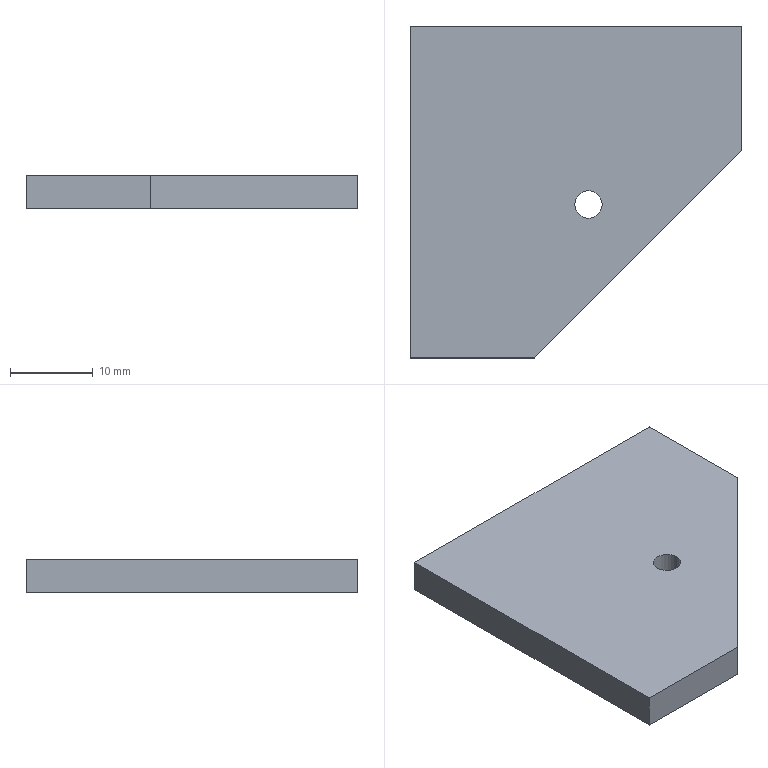Part | STEP file | PN_0073 sheet-metal fixing block | 1 solid | 9 faces | box 40 x 40 x 4 mm | volume 5116 mm3 | plane 7 | cylinder 2 | commonest cylinder face diameters 3.3 x2
STEP:
#1=CARTESIAN_POINT('',(0.,0.,0.));
#2=DIRECTION('',(0.,0.,1.));
#3=DIRECTION('',(1.,0.,0.));
#4=AXIS2_PLACEMENT_3D('',#1,#2,#3);
#5=CARTESIAN_POINT('',(23.15,-21.5,-2.));
#6=VERTEX_POINT('',#5);
#7=CARTESIAN_POINT('',(23.15,-21.5,2.));
#8=VERTEX_POINT('',#7);
#9=CARTESIAN_POINT('',(23.15,-21.5,2.));
#10=DIRECTION('',(0.,0.,1.));
#11=VECTOR('',#10,1.);
#12=LINE('',#9,#11);
#13=CARTESIAN_POINT('',(21.5,-21.5,2.));
#14=DIRECTION('',(0.,0.,1.));
#15=DIRECTION('',(1.,0.,0.));
#16=AXIS2_PLACEMENT_3D('',#13,#14,#15);
#17=CYLINDRICAL_SURFACE('',#16,1.65);
#18=CARTESIAN_POINT('',(6.283,0.));
#19=DIRECTION('',(0.,1.));
#20=VECTOR('',#19,1.);
#21=LINE('',#18,#20);
#22=(GEOMETRIC_REPRESENTATION_CONTEXT(2)PARAMETRIC_REPRESENTATION_CONTEXT()REPRESENTATION_CONTEXT('',''));
#23=DEFINITIONAL_REPRESENTATION('',(#21),#22);
#24=PCURVE('',#17,#23);
#25=CARTESIAN_POINT('',(21.5,-21.5,2.));
#26=DIRECTION('',(0.,0.,1.));
#27=DIRECTION('',(1.,0.,0.));
#28=AXIS2_PLACEMENT_3D('',#25,#26,#27);
#29=CYLINDRICAL_SURFACE('',#28,1.65);
#30=CARTESIAN_POINT('',(0.,0.));
#31=DIRECTION('',(0.,1.));
#32=VECTOR('',#31,1.);
#33=LINE('',#30,#32);
#34=(GEOMETRIC_REPRESENTATION_CONTEXT(2)PARAMETRIC_REPRESENTATION_CONTEXT()REPRESENTATION_CONTEXT('',''));
#35=DEFINITIONAL_REPRESENTATION('',(#33),#34);
#36=PCURVE('',#29,#35);
#37=SURFACE_CURVE('',#12,(#24,#36),.PCURVE_S1.);
#38=EDGE_CURVE('',#6,#8,#37,.T.);
#39=ORIENTED_EDGE('',*,*,#38,.T.);
#40=CARTESIAN_POINT('',(19.85,-21.5,2.));
#41=VERTEX_POINT('',#40);
#42=CARTESIAN_POINT('',(21.5,-21.5,2.));
#43=DIRECTION('',(0.,0.,1.));
#44=DIRECTION('',(1.,0.,0.));
#45=AXIS2_PLACEMENT_3D('',#42,#43,#44);
#46=CIRCLE('',#45,1.65);
#47=CARTESIAN_POINT('',(0.,0.));
#48=DIRECTION('',(1.,0.));
#49=VECTOR('',#48,1.);
#50=LINE('',#47,#49);
#51=(GEOMETRIC_REPRESENTATION_CONTEXT(2)PARAMETRIC_REPRESENTATION_CONTEXT()REPRESENTATION_CONTEXT('',''));
#52=DEFINITIONAL_REPRESENTATION('',(#50),#51);
#53=PCURVE('',#17,#52);
#54=CARTESIAN_POINT('',(0.,0.,2.));
#55=DIRECTION('',(0.,0.,1.));
#56=DIRECTION('',(1.,0.,0.));
#57=AXIS2_PLACEMENT_3D('',#54,#55,#56);
#58=PLANE('',#57);
#59=CARTESIAN_POINT('',(21.5,-21.5));
#60=DIRECTION('',(1.,0.));
#61=AXIS2_PLACEMENT_2D('',#59,#60);
#62=CIRCLE('',#61,1.65);
#63=(GEOMETRIC_REPRESENTATION_CONTEXT(2)PARAMETRIC_REPRESENTATION_CONTEXT()REPRESENTATION_CONTEXT('',''));
#64=DEFINITIONAL_REPRESENTATION('',(#62),#63);
#65=PCURVE('',#58,#64);
#66=SURFACE_CURVE('',#46,(#53,#65),.PCURVE_S1.);
#67=EDGE_CURVE('',#41,#8,#66,.T.);
#68=ORIENTED_EDGE('',*,*,#67,.F.);
#69=CARTESIAN_POINT('',(19.85,-21.5,-2.));
#70=VERTEX_POINT('',#69);
#71=CARTESIAN_POINT('',(19.85,-21.5,2.));
#72=DIRECTION('',(0.,0.,1.));
#73=VECTOR('',#72,1.);
#74=LINE('',#71,#73);
#75=CARTESIAN_POINT('',(3.142,0.));
#76=DIRECTION('',(0.,1.));
#77=VECTOR('',#76,1.);
#78=LINE('',#75,#77);
#79=(GEOMETRIC_REPRESENTATION_CONTEXT(2)PARAMETRIC_REPRESENTATION_CONTEXT()REPRESENTATION_CONTEXT('',''));
#80=DEFINITIONAL_REPRESENTATION('',(#78),#79);
#81=PCURVE('',#17,#80);
#82=CARTESIAN_POINT('',(3.142,0.));
#83=DIRECTION('',(0.,1.));
#84=VECTOR('',#83,1.);
#85=LINE('',#82,#84);
#86=(GEOMETRIC_REPRESENTATION_CONTEXT(2)PARAMETRIC_REPRESENTATION_CONTEXT()REPRESENTATION_CONTEXT('',''));
#87=DEFINITIONAL_REPRESENTATION('',(#85),#86);
#88=PCURVE('',#29,#87);
#89=SURFACE_CURVE('',#74,(#81,#88),.PCURVE_S1.);
#90=EDGE_CURVE('',#70,#41,#89,.T.);
#91=ORIENTED_EDGE('',*,*,#90,.F.);
#92=CARTESIAN_POINT('',(21.5,-21.5,-2.));
#93=DIRECTION('',(0.,0.,1.));
#94=DIRECTION('',(1.,0.,0.));
#95=AXIS2_PLACEMENT_3D('',#92,#93,#94);
#96=CIRCLE('',#95,1.65);
#97=CARTESIAN_POINT('',(0.,-4.));
#98=DIRECTION('',(1.,0.));
#99=VECTOR('',#98,1.);
#100=LINE('',#97,#99);
#101=(GEOMETRIC_REPRESENTATION_CONTEXT(2)PARAMETRIC_REPRESENTATION_CONTEXT()REPRESENTATION_CONTEXT('',''));
#102=DEFINITIONAL_REPRESENTATION('',(#100),#101);
#103=PCURVE('',#17,#102);
#104=CARTESIAN_POINT('',(0.,0.,-2.));
#105=DIRECTION('',(0.,0.,1.));
#106=DIRECTION('',(1.,0.,0.));
#107=AXIS2_PLACEMENT_3D('',#104,#105,#106);
#108=PLANE('',#107);
#109=CARTESIAN_POINT('',(21.5,-21.5));
#110=DIRECTION('',(1.,0.));
#111=AXIS2_PLACEMENT_2D('',#109,#110);
#112=CIRCLE('',#111,1.65);
#113=(GEOMETRIC_REPRESENTATION_CONTEXT(2)PARAMETRIC_REPRESENTATION_CONTEXT()REPRESENTATION_CONTEXT('',''));
#114=DEFINITIONAL_REPRESENTATION('',(#112),#113);
#115=PCURVE('',#108,#114);
#116=SURFACE_CURVE('',#96,(#103,#115),.PCURVE_S1.);
#117=EDGE_CURVE('',#70,#6,#116,.T.);
#118=ORIENTED_EDGE('',*,*,#117,.T.);
#119=EDGE_LOOP('',(#39,#68,#91,#118));
#120=FACE_BOUND('',#119,.F.);
#121=ADVANCED_FACE('',(#120),#17,.F.);
#122=CARTESIAN_POINT('',(0.,0.,-2.));
#123=VERTEX_POINT('',#122);
#124=CARTESIAN_POINT('',(0.,-40.,-2.));
#125=VERTEX_POINT('',#124);
#126=CARTESIAN_POINT('',(0.,0.,-2.));
#127=DIRECTION('',(0.,-1.,0.));
#128=VECTOR('',#127,1.);
#129=LINE('',#126,#128);
#130=CARTESIAN_POINT('',(0.,0.,2.));
#131=DIRECTION('',(1.,0.,0.));
#132=DIRECTION('',(0.,1.,0.));
#133=AXIS2_PLACEMENT_3D('',#130,#131,#132);
#134=PLANE('',#133);
#135=CARTESIAN_POINT('',(0.,-4.));
#136=DIRECTION('',(-1.,0.));
#137=VECTOR('',#136,1.);
#138=LINE('',#135,#137);
#139=(GEOMETRIC_REPRESENTATION_CONTEXT(2)PARAMETRIC_REPRESENTATION_CONTEXT()REPRESENTATION_CONTEXT('',''));
#140=DEFINITIONAL_REPRESENTATION('',(#138),#139);
#141=PCURVE('',#134,#140);
#142=CARTESIAN_POINT('',(0.,0.));
#143=DIRECTION('',(0.,-1.));
#144=VECTOR('',#143,1.);
#145=LINE('',#142,#144);
#146=(GEOMETRIC_REPRESENTATION_CONTEXT(2)PARAMETRIC_REPRESENTATION_CONTEXT()REPRESENTATION_CONTEXT('',''));
#147=DEFINITIONAL_REPRESENTATION('',(#145),#146);
#148=PCURVE('',#108,#147);
#149=SURFACE_CURVE('',#129,(#141,#148),.PCURVE_S1.);
#150=EDGE_CURVE('',#123,#125,#149,.T.);
#151=ORIENTED_EDGE('',*,*,#150,.T.);
#152=CARTESIAN_POINT('',(0.,-40.,2.));
#153=VERTEX_POINT('',#152);
#154=CARTESIAN_POINT('',(0.,-40.,2.));
#155=DIRECTION('',(0.,0.,-1.));
#156=VECTOR('',#155,1.);
#157=LINE('',#154,#156);
#158=CARTESIAN_POINT('',(-40.,0.));
#159=DIRECTION('',(0.,-1.));
#160=VECTOR('',#159,1.);
#161=LINE('',#158,#160);
#162=(GEOMETRIC_REPRESENTATION_CONTEXT(2)PARAMETRIC_REPRESENTATION_CONTEXT()REPRESENTATION_CONTEXT('',''));
#163=DEFINITIONAL_REPRESENTATION('',(#161),#162);
#164=PCURVE('',#134,#163);
#165=CARTESIAN_POINT('',(0.,-40.,2.));
#166=DIRECTION('',(0.,1.,0.));
#167=DIRECTION('',(0.,0.,1.));
#168=AXIS2_PLACEMENT_3D('',#165,#166,#167);
#169=PLANE('',#168);
#170=CARTESIAN_POINT('',(0.,0.));
#171=DIRECTION('',(-1.,0.));
#172=VECTOR('',#171,1.);
#173=LINE('',#170,#172);
#174=(GEOMETRIC_REPRESENTATION_CONTEXT(2)PARAMETRIC_REPRESENTATION_CONTEXT()REPRESENTATION_CONTEXT('',''));
#175=DEFINITIONAL_REPRESENTATION('',(#173),#174);
#176=PCURVE('',#169,#175);
#177=SURFACE_CURVE('',#157,(#164,#176),.PCURVE_S1.);
#178=EDGE_CURVE('',#153,#125,#177,.T.);
#179=ORIENTED_EDGE('',*,*,#178,.F.);
#180=CARTESIAN_POINT('',(0.,0.,2.));
#181=VERTEX_POINT('',#180);
#182=CARTESIAN_POINT('',(0.,0.,2.));
#183=DIRECTION('',(0.,-1.,0.));
#184=VECTOR('',#183,1.);
#185=LINE('',#182,#184);
#186=CARTESIAN_POINT('',(0.,0.));
#187=DIRECTION('',(-1.,0.));
#188=VECTOR('',#187,1.);
#189=LINE('',#186,#188);
#190=(GEOMETRIC_REPRESENTATION_CONTEXT(2)PARAMETRIC_REPRESENTATION_CONTEXT()REPRESENTATION_CONTEXT('',''));
#191=DEFINITIONAL_REPRESENTATION('',(#189),#190);
#192=PCURVE('',#134,#191);
#193=CARTESIAN_POINT('',(0.,0.));
#194=DIRECTION('',(0.,-1.));
#195=VECTOR('',#194,1.);
#196=LINE('',#193,#195);
#197=(GEOMETRIC_REPRESENTATION_CONTEXT(2)PARAMETRIC_REPRESENTATION_CONTEXT()REPRESENTATION_CONTEXT('',''));
#198=DEFINITIONAL_REPRESENTATION('',(#196),#197);
#199=PCURVE('',#58,#198);
#200=SURFACE_CURVE('',#185,(#192,#199),.PCURVE_S1.);
#201=EDGE_CURVE('',#181,#153,#200,.T.);
#202=ORIENTED_EDGE('',*,*,#201,.F.);
#203=CARTESIAN_POINT('',(0.,0.,2.));
#204=DIRECTION('',(0.,0.,-1.));
#205=VECTOR('',#204,1.);
#206=LINE('',#203,#205);
#207=CARTESIAN_POINT('',(0.,0.));
#208=DIRECTION('',(0.,-1.));
#209=VECTOR('',#208,1.);
#210=LINE('',#207,#209);
#211=(GEOMETRIC_REPRESENTATION_CONTEXT(2)PARAMETRIC_REPRESENTATION_CONTEXT()REPRESENTATION_CONTEXT('',''));
#212=DEFINITIONAL_REPRESENTATION('',(#210),#211);
#213=PCURVE('',#134,#212);
#214=CARTESIAN_POINT('',(0.,0.,2.));
#215=DIRECTION('',(0.,-1.,0.));
#216=DIRECTION('',(0.,0.,-1.));
#217=AXIS2_PLACEMENT_3D('',#214,#215,#216);
#218=PLANE('',#217);
#219=CARTESIAN_POINT('',(0.,0.));
#220=DIRECTION('',(1.,0.));
#221=VECTOR('',#220,1.);
#222=LINE('',#219,#221);
#223=(GEOMETRIC_REPRESENTATION_CONTEXT(2)PARAMETRIC_REPRESENTATION_CONTEXT()REPRESENTATION_CONTEXT('',''));
#224=DEFINITIONAL_REPRESENTATION('',(#222),#223);
#225=PCURVE('',#218,#224);
#226=SURFACE_CURVE('',#206,(#213,#225),.PCURVE_S1.);
#227=EDGE_CURVE('',#181,#123,#226,.T.);
#228=ORIENTED_EDGE('',*,*,#227,.T.);
#229=EDGE_LOOP('',(#151,#179,#202,#228));
#230=FACE_BOUND('',#229,.T.);
#231=ADVANCED_FACE('',(#230),#134,.F.);
#232=CARTESIAN_POINT('',(15.,-40.,-2.));
#233=VERTEX_POINT('',#232);
#234=CARTESIAN_POINT('',(0.,-40.,-2.));
#235=DIRECTION('',(1.,0.,0.));
#236=VECTOR('',#235,1.);
#237=LINE('',#234,#236);
#238=CARTESIAN_POINT('',(-4.,0.));
#239=DIRECTION('',(0.,1.));
#240=VECTOR('',#239,1.);
#241=LINE('',#238,#240);
#242=(GEOMETRIC_REPRESENTATION_CONTEXT(2)PARAMETRIC_REPRESENTATION_CONTEXT()REPRESENTATION_CONTEXT('',''));
#243=DEFINITIONAL_REPRESENTATION('',(#241),#242);
#244=PCURVE('',#169,#243);
#245=CARTESIAN_POINT('',(0.,-40.));
#246=DIRECTION('',(1.,0.));
#247=VECTOR('',#246,1.);
#248=LINE('',#245,#247);
#249=(GEOMETRIC_REPRESENTATION_CONTEXT(2)PARAMETRIC_REPRESENTATION_CONTEXT()REPRESENTATION_CONTEXT('',''));
#250=DEFINITIONAL_REPRESENTATION('',(#248),#249);
#251=PCURVE('',#108,#250);
#252=SURFACE_CURVE('',#237,(#244,#251),.PCURVE_S1.);
#253=EDGE_CURVE('',#125,#233,#252,.T.);
#254=ORIENTED_EDGE('',*,*,#253,.T.);
#255=CARTESIAN_POINT('',(15.,-40.,2.));
#256=VERTEX_POINT('',#255);
#257=CARTESIAN_POINT('',(15.,-40.,2.));
#258=DIRECTION('',(0.,0.,-1.));
#259=VECTOR('',#258,1.);
#260=LINE('',#257,#259);
#261=CARTESIAN_POINT('',(0.,15.));
#262=DIRECTION('',(-1.,0.));
#263=VECTOR('',#262,1.);
#264=LINE('',#261,#263);
#265=(GEOMETRIC_REPRESENTATION_CONTEXT(2)PARAMETRIC_REPRESENTATION_CONTEXT()REPRESENTATION_CONTEXT('',''));
#266=DEFINITIONAL_REPRESENTATION('',(#264),#265);
#267=PCURVE('',#169,#266);
#268=CARTESIAN_POINT('',(15.,-40.,2.));
#269=DIRECTION('',(-0.7071,0.7071,0.));
#270=DIRECTION('',(-0.7071,-0.7071,0.));
#271=AXIS2_PLACEMENT_3D('',#268,#269,#270);
#272=PLANE('',#271);
#273=CARTESIAN_POINT('',(0.,0.));
#274=DIRECTION('',(0.,-1.));
#275=VECTOR('',#274,1.);
#276=LINE('',#273,#275);
#277=(GEOMETRIC_REPRESENTATION_CONTEXT(2)PARAMETRIC_REPRESENTATION_CONTEXT()REPRESENTATION_CONTEXT('',''));
#278=DEFINITIONAL_REPRESENTATION('',(#276),#277);
#279=PCURVE('',#272,#278);
#280=SURFACE_CURVE('',#260,(#267,#279),.PCURVE_S1.);
#281=EDGE_CURVE('',#256,#233,#280,.T.);
#282=ORIENTED_EDGE('',*,*,#281,.F.);
#283=CARTESIAN_POINT('',(0.,-40.,2.));
#284=DIRECTION('',(1.,0.,0.));
#285=VECTOR('',#284,1.);
#286=LINE('',#283,#285);
#287=CARTESIAN_POINT('',(0.,0.));
#288=DIRECTION('',(0.,1.));
#289=VECTOR('',#288,1.);
#290=LINE('',#287,#289);
#291=(GEOMETRIC_REPRESENTATION_CONTEXT(2)PARAMETRIC_REPRESENTATION_CONTEXT()REPRESENTATION_CONTEXT('',''));
#292=DEFINITIONAL_REPRESENTATION('',(#290),#291);
#293=PCURVE('',#169,#292);
#294=CARTESIAN_POINT('',(0.,-40.));
#295=DIRECTION('',(1.,0.));
#296=VECTOR('',#295,1.);
#297=LINE('',#294,#296);
#298=(GEOMETRIC_REPRESENTATION_CONTEXT(2)PARAMETRIC_REPRESENTATION_CONTEXT()REPRESENTATION_CONTEXT('',''));
#299=DEFINITIONAL_REPRESENTATION('',(#297),#298);
#300=PCURVE('',#58,#299);
#301=SURFACE_CURVE('',#286,(#293,#300),.PCURVE_S1.);
#302=EDGE_CURVE('',#153,#256,#301,.T.);
#303=ORIENTED_EDGE('',*,*,#302,.F.);
#304=ORIENTED_EDGE('',*,*,#178,.T.);
#305=EDGE_LOOP('',(#254,#282,#303,#304));
#306=FACE_BOUND('',#305,.T.);
#307=ADVANCED_FACE('',(#306),#169,.F.);
#308=CARTESIAN_POINT('',(40.,-15.,-2.));
#309=VERTEX_POINT('',#308);
#310=CARTESIAN_POINT('',(15.,-40.,-2.));
#311=DIRECTION('',(0.7071,0.7071,0.));
#312=VECTOR('',#311,1.);
#313=LINE('',#310,#312);
#314=CARTESIAN_POINT('',(0.,-4.));
#315=DIRECTION('',(-1.,0.));
#316=VECTOR('',#315,1.);
#317=LINE('',#314,#316);
#318=(GEOMETRIC_REPRESENTATION_CONTEXT(2)PARAMETRIC_REPRESENTATION_CONTEXT()REPRESENTATION_CONTEXT('',''));
#319=DEFINITIONAL_REPRESENTATION('',(#317),#318);
#320=PCURVE('',#272,#319);
#321=CARTESIAN_POINT('',(15.,-40.));
#322=DIRECTION('',(0.7071,0.7071));
#323=VECTOR('',#322,1.);
#324=LINE('',#321,#323);
#325=(GEOMETRIC_REPRESENTATION_CONTEXT(2)PARAMETRIC_REPRESENTATION_CONTEXT()REPRESENTATION_CONTEXT('',''));
#326=DEFINITIONAL_REPRESENTATION('',(#324),#325);
#327=PCURVE('',#108,#326);
#328=SURFACE_CURVE('',#313,(#320,#327),.PCURVE_S1.);
#329=EDGE_CURVE('',#233,#309,#328,.T.);
#330=ORIENTED_EDGE('',*,*,#329,.T.);
#331=CARTESIAN_POINT('',(40.,-15.,2.));
#332=VERTEX_POINT('',#331);
#333=CARTESIAN_POINT('',(40.,-15.,2.));
#334=DIRECTION('',(0.,0.,-1.));
#335=VECTOR('',#334,1.);
#336=LINE('',#333,#335);
#337=CARTESIAN_POINT('',(-35.355,0.));
#338=DIRECTION('',(0.,-1.));
#339=VECTOR('',#338,1.);
#340=LINE('',#337,#339);
#341=(GEOMETRIC_REPRESENTATION_CONTEXT(2)PARAMETRIC_REPRESENTATION_CONTEXT()REPRESENTATION_CONTEXT('',''));
#342=DEFINITIONAL_REPRESENTATION('',(#340),#341);
#343=PCURVE('',#272,#342);
#344=CARTESIAN_POINT('',(40.,0.,2.));
#345=DIRECTION('',(-1.,0.,0.));
#346=DIRECTION('',(0.,0.,1.));
#347=AXIS2_PLACEMENT_3D('',#344,#345,#346);
#348=PLANE('',#347);
#349=CARTESIAN_POINT('',(0.,-15.));
#350=DIRECTION('',(-1.,0.));
#351=VECTOR('',#350,1.);
#352=LINE('',#349,#351);
#353=(GEOMETRIC_REPRESENTATION_CONTEXT(2)PARAMETRIC_REPRESENTATION_CONTEXT()REPRESENTATION_CONTEXT('',''));
#354=DEFINITIONAL_REPRESENTATION('',(#352),#353);
#355=PCURVE('',#348,#354);
#356=SURFACE_CURVE('',#336,(#343,#355),.PCURVE_S1.);
#357=EDGE_CURVE('',#332,#309,#356,.T.);
#358=ORIENTED_EDGE('',*,*,#357,.F.);
#359=CARTESIAN_POINT('',(15.,-40.,2.));
#360=DIRECTION('',(0.7071,0.7071,0.));
#361=VECTOR('',#360,1.);
#362=LINE('',#359,#361);
#363=CARTESIAN_POINT('',(0.,0.));
#364=DIRECTION('',(-1.,0.));
#365=VECTOR('',#364,1.);
#366=LINE('',#363,#365);
#367=(GEOMETRIC_REPRESENTATION_CONTEXT(2)PARAMETRIC_REPRESENTATION_CONTEXT()REPRESENTATION_CONTEXT('',''));
#368=DEFINITIONAL_REPRESENTATION('',(#366),#367);
#369=PCURVE('',#272,#368);
#370=CARTESIAN_POINT('',(15.,-40.));
#371=DIRECTION('',(0.7071,0.7071));
#372=VECTOR('',#371,1.);
#373=LINE('',#370,#372);
#374=(GEOMETRIC_REPRESENTATION_CONTEXT(2)PARAMETRIC_REPRESENTATION_CONTEXT()REPRESENTATION_CONTEXT('',''));
#375=DEFINITIONAL_REPRESENTATION('',(#373),#374);
#376=PCURVE('',#58,#375);
#377=SURFACE_CURVE('',#362,(#369,#376),.PCURVE_S1.);
#378=EDGE_CURVE('',#256,#332,#377,.T.);
#379=ORIENTED_EDGE('',*,*,#378,.F.);
#380=ORIENTED_EDGE('',*,*,#281,.T.);
#381=EDGE_LOOP('',(#330,#358,#379,#380));
#382=FACE_BOUND('',#381,.T.);
#383=ADVANCED_FACE('',(#382),#272,.F.);
#384=CARTESIAN_POINT('',(40.,0.,-2.));
#385=VERTEX_POINT('',#384);
#386=CARTESIAN_POINT('',(40.,0.,-2.));
#387=DIRECTION('',(0.,1.,0.));
#388=VECTOR('',#387,1.);
#389=LINE('',#386,#388);
#390=CARTESIAN_POINT('',(-4.,0.));
#391=DIRECTION('',(0.,1.));
#392=VECTOR('',#391,1.);
#393=LINE('',#390,#392);
#394=(GEOMETRIC_REPRESENTATION_CONTEXT(2)PARAMETRIC_REPRESENTATION_CONTEXT()REPRESENTATION_CONTEXT('',''));
#395=DEFINITIONAL_REPRESENTATION('',(#393),#394);
#396=PCURVE('',#348,#395);
#397=CARTESIAN_POINT('',(40.,0.));
#398=DIRECTION('',(0.,1.));
#399=VECTOR('',#398,1.);
#400=LINE('',#397,#399);
#401=(GEOMETRIC_REPRESENTATION_CONTEXT(2)PARAMETRIC_REPRESENTATION_CONTEXT()REPRESENTATION_CONTEXT('',''));
#402=DEFINITIONAL_REPRESENTATION('',(#400),#401);
#403=PCURVE('',#108,#402);
#404=SURFACE_CURVE('',#389,(#396,#403),.PCURVE_S1.);
#405=EDGE_CURVE('',#309,#385,#404,.T.);
#406=ORIENTED_EDGE('',*,*,#405,.T.);
#407=CARTESIAN_POINT('',(40.,0.,2.));
#408=VERTEX_POINT('',#407);
#409=CARTESIAN_POINT('',(40.,0.,2.));
#410=DIRECTION('',(0.,0.,-1.));
#411=VECTOR('',#410,1.);
#412=LINE('',#409,#411);
#413=CARTESIAN_POINT('',(0.,0.));
#414=DIRECTION('',(-1.,0.));
#415=VECTOR('',#414,1.);
#416=LINE('',#413,#415);
#417=(GEOMETRIC_REPRESENTATION_CONTEXT(2)PARAMETRIC_REPRESENTATION_CONTEXT()REPRESENTATION_CONTEXT('',''));
#418=DEFINITIONAL_REPRESENTATION('',(#416),#417);
#419=PCURVE('',#348,#418);
#420=CARTESIAN_POINT('',(0.,40.));
#421=DIRECTION('',(1.,0.));
#422=VECTOR('',#421,1.);
#423=LINE('',#420,#422);
#424=(GEOMETRIC_REPRESENTATION_CONTEXT(2)PARAMETRIC_REPRESENTATION_CONTEXT()REPRESENTATION_CONTEXT('',''));
#425=DEFINITIONAL_REPRESENTATION('',(#423),#424);
#426=PCURVE('',#218,#425);
#427=SURFACE_CURVE('',#412,(#419,#426),.PCURVE_S1.);
#428=EDGE_CURVE('',#408,#385,#427,.T.);
#429=ORIENTED_EDGE('',*,*,#428,.F.);
#430=CARTESIAN_POINT('',(40.,0.,2.));
#431=DIRECTION('',(0.,1.,0.));
#432=VECTOR('',#431,1.);
#433=LINE('',#430,#432);
#434=CARTESIAN_POINT('',(0.,0.));
#435=DIRECTION('',(0.,1.));
#436=VECTOR('',#435,1.);
#437=LINE('',#434,#436);
#438=(GEOMETRIC_REPRESENTATION_CONTEXT(2)PARAMETRIC_REPRESENTATION_CONTEXT()REPRESENTATION_CONTEXT('',''));
#439=DEFINITIONAL_REPRESENTATION('',(#437),#438);
#440=PCURVE('',#348,#439);
#441=CARTESIAN_POINT('',(40.,0.));
#442=DIRECTION('',(0.,1.));
#443=VECTOR('',#442,1.);
#444=LINE('',#441,#443);
#445=(GEOMETRIC_REPRESENTATION_CONTEXT(2)PARAMETRIC_REPRESENTATION_CONTEXT()REPRESENTATION_CONTEXT('',''));
#446=DEFINITIONAL_REPRESENTATION('',(#444),#445);
#447=PCURVE('',#58,#446);
#448=SURFACE_CURVE('',#433,(#440,#447),.PCURVE_S1.);
#449=EDGE_CURVE('',#332,#408,#448,.T.);
#450=ORIENTED_EDGE('',*,*,#449,.F.);
#451=ORIENTED_EDGE('',*,*,#357,.T.);
#452=EDGE_LOOP('',(#406,#429,#450,#451));
#453=FACE_BOUND('',#452,.T.);
#454=ADVANCED_FACE('',(#453),#348,.F.);
#455=CARTESIAN_POINT('',(0.,0.,-2.));
#456=DIRECTION('',(-1.,0.,0.));
#457=VECTOR('',#456,1.);
#458=LINE('',#455,#457);
#459=CARTESIAN_POINT('',(4.,0.));
#460=DIRECTION('',(0.,-1.));
#461=VECTOR('',#460,1.);
#462=LINE('',#459,#461);
#463=(GEOMETRIC_REPRESENTATION_CONTEXT(2)PARAMETRIC_REPRESENTATION_CONTEXT()REPRESENTATION_CONTEXT('',''));
#464=DEFINITIONAL_REPRESENTATION('',(#462),#463);
#465=PCURVE('',#218,#464);
#466=CARTESIAN_POINT('',(0.,0.));
#467=DIRECTION('',(-1.,0.));
#468=VECTOR('',#467,1.);
#469=LINE('',#466,#468);
#470=(GEOMETRIC_REPRESENTATION_CONTEXT(2)PARAMETRIC_REPRESENTATION_CONTEXT()REPRESENTATION_CONTEXT('',''));
#471=DEFINITIONAL_REPRESENTATION('',(#469),#470);
#472=PCURVE('',#108,#471);
#473=SURFACE_CURVE('',#458,(#465,#472),.PCURVE_S1.);
#474=EDGE_CURVE('',#385,#123,#473,.T.);
#475=ORIENTED_EDGE('',*,*,#474,.T.);
#476=ORIENTED_EDGE('',*,*,#227,.F.);
#477=CARTESIAN_POINT('',(0.,0.,2.));
#478=DIRECTION('',(-1.,0.,0.));
#479=VECTOR('',#478,1.);
#480=LINE('',#477,#479);
#481=CARTESIAN_POINT('',(0.,0.));
#482=DIRECTION('',(0.,-1.));
#483=VECTOR('',#482,1.);
#484=LINE('',#481,#483);
#485=(GEOMETRIC_REPRESENTATION_CONTEXT(2)PARAMETRIC_REPRESENTATION_CONTEXT()REPRESENTATION_CONTEXT('',''));
#486=DEFINITIONAL_REPRESENTATION('',(#484),#485);
#487=PCURVE('',#218,#486);
#488=CARTESIAN_POINT('',(0.,0.));
#489=DIRECTION('',(-1.,0.));
#490=VECTOR('',#489,1.);
#491=LINE('',#488,#490);
#492=(GEOMETRIC_REPRESENTATION_CONTEXT(2)PARAMETRIC_REPRESENTATION_CONTEXT()REPRESENTATION_CONTEXT('',''));
#493=DEFINITIONAL_REPRESENTATION('',(#491),#492);
#494=PCURVE('',#58,#493);
#495=SURFACE_CURVE('',#480,(#487,#494),.PCURVE_S1.);
#496=EDGE_CURVE('',#408,#181,#495,.T.);
#497=ORIENTED_EDGE('',*,*,#496,.F.);
#498=ORIENTED_EDGE('',*,*,#428,.T.);
#499=EDGE_LOOP('',(#475,#476,#497,#498));
#500=FACE_BOUND('',#499,.T.);
#501=ADVANCED_FACE('',(#500),#218,.F.);
#502=CARTESIAN_POINT('',(21.5,-21.5,2.));
#503=DIRECTION('',(0.,0.,1.));
#504=DIRECTION('',(1.,0.,0.));
#505=AXIS2_PLACEMENT_3D('',#502,#503,#504);
#506=CIRCLE('',#505,1.65);
#507=CARTESIAN_POINT('',(21.5,-21.5));
#508=DIRECTION('',(1.,0.));
#509=AXIS2_PLACEMENT_2D('',#507,#508);
#510=CIRCLE('',#509,1.65);
#511=(GEOMETRIC_REPRESENTATION_CONTEXT(2)PARAMETRIC_REPRESENTATION_CONTEXT()REPRESENTATION_CONTEXT('',''));
#512=DEFINITIONAL_REPRESENTATION('',(#510),#511);
#513=PCURVE('',#58,#512);
#514=CARTESIAN_POINT('',(0.,0.));
#515=DIRECTION('',(1.,0.));
#516=VECTOR('',#515,1.);
#517=LINE('',#514,#516);
#518=(GEOMETRIC_REPRESENTATION_CONTEXT(2)PARAMETRIC_REPRESENTATION_CONTEXT()REPRESENTATION_CONTEXT('',''));
#519=DEFINITIONAL_REPRESENTATION('',(#517),#518);
#520=PCURVE('',#29,#519);
#521=SURFACE_CURVE('',#506,(#513,#520),.PCURVE_S1.);
#522=EDGE_CURVE('',#8,#41,#521,.T.);
#523=ORIENTED_EDGE('',*,*,#522,.F.);
#524=ORIENTED_EDGE('',*,*,#67,.F.);
#525=EDGE_LOOP('',(#523,#524));
#526=FACE_BOUND('',#525,.T.);
#527=ORIENTED_EDGE('',*,*,#201,.T.);
#528=ORIENTED_EDGE('',*,*,#302,.T.);
#529=ORIENTED_EDGE('',*,*,#378,.T.);
#530=ORIENTED_EDGE('',*,*,#449,.T.);
#531=ORIENTED_EDGE('',*,*,#496,.T.);
#532=EDGE_LOOP('',(#527,#528,#529,#530,#531));
#533=FACE_BOUND('',#532,.T.);
#534=ADVANCED_FACE('',(#526,#533),#58,.T.);
#535=CARTESIAN_POINT('',(21.5,-21.5,-2.));
#536=DIRECTION('',(0.,0.,1.));
#537=DIRECTION('',(1.,0.,0.));
#538=AXIS2_PLACEMENT_3D('',#535,#536,#537);
#539=CIRCLE('',#538,1.65);
#540=CARTESIAN_POINT('',(21.5,-21.5));
#541=DIRECTION('',(1.,0.));
#542=AXIS2_PLACEMENT_2D('',#540,#541);
#543=CIRCLE('',#542,1.65);
#544=(GEOMETRIC_REPRESENTATION_CONTEXT(2)PARAMETRIC_REPRESENTATION_CONTEXT()REPRESENTATION_CONTEXT('',''));
#545=DEFINITIONAL_REPRESENTATION('',(#543),#544);
#546=PCURVE('',#108,#545);
#547=CARTESIAN_POINT('',(0.,-4.));
#548=DIRECTION('',(1.,0.));
#549=VECTOR('',#548,1.);
#550=LINE('',#547,#549);
#551=(GEOMETRIC_REPRESENTATION_CONTEXT(2)PARAMETRIC_REPRESENTATION_CONTEXT()REPRESENTATION_CONTEXT('',''));
#552=DEFINITIONAL_REPRESENTATION('',(#550),#551);
#553=PCURVE('',#29,#552);
#554=SURFACE_CURVE('',#539,(#546,#553),.PCURVE_S1.);
#555=EDGE_CURVE('',#6,#70,#554,.T.);
#556=ORIENTED_EDGE('',*,*,#555,.T.);
#557=ORIENTED_EDGE('',*,*,#117,.T.);
#558=EDGE_LOOP('',(#556,#557));
#559=FACE_BOUND('',#558,.T.);
#560=ORIENTED_EDGE('',*,*,#150,.F.);
#561=ORIENTED_EDGE('',*,*,#474,.F.);
#562=ORIENTED_EDGE('',*,*,#405,.F.);
#563=ORIENTED_EDGE('',*,*,#329,.F.);
#564=ORIENTED_EDGE('',*,*,#253,.F.);
#565=EDGE_LOOP('',(#560,#561,#562,#563,#564));
#566=FACE_BOUND('',#565,.T.);
#567=ADVANCED_FACE('',(#559,#566),#108,.F.);
#568=ORIENTED_EDGE('',*,*,#522,.F.);
#569=ORIENTED_EDGE('',*,*,#38,.F.);
#570=ORIENTED_EDGE('',*,*,#555,.T.);
#571=ORIENTED_EDGE('',*,*,#90,.T.);
#572=EDGE_LOOP('',(#568,#569,#570,#571));
#573=FACE_BOUND('',#572,.F.);
#574=ADVANCED_FACE('',(#573),#29,.F.);
#575=CLOSED_SHELL('',(#121,#231,#307,#383,#454,#501,#534,#567,#574));
#576=MANIFOLD_SOLID_BREP('',#575);
#577=(LENGTH_UNIT()NAMED_UNIT(*)SI_UNIT(.MILLI.,.METRE.));
#578=UNCERTAINTY_MEASURE_WITH_UNIT(LENGTH_MEASURE(0.0000001),#577,'','');
#579=(NAMED_UNIT(*)PLANE_ANGLE_UNIT()SI_UNIT($,.RADIAN.));
#580=(NAMED_UNIT(*)SI_UNIT($,.STERADIAN.)SOLID_ANGLE_UNIT());
#581=(GEOMETRIC_REPRESENTATION_CONTEXT(3)GLOBAL_UNCERTAINTY_ASSIGNED_CONTEXT((#578))GLOBAL_UNIT_ASSIGNED_CONTEXT((#577,#579,#580))REPRESENTATION_CONTEXT('',''));
#582=ADVANCED_BREP_SHAPE_REPRESENTATION('',(#4,#576),#581);